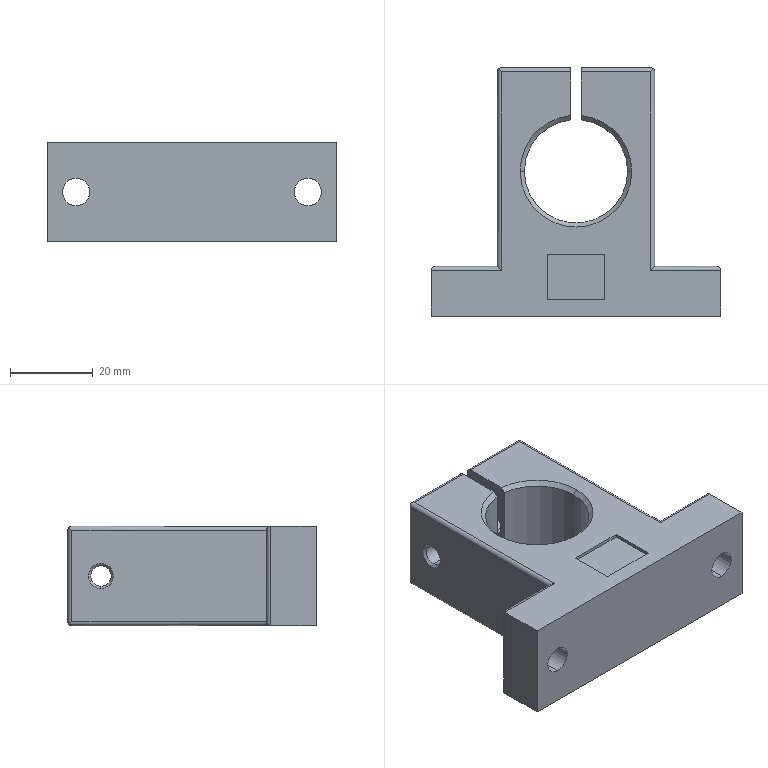Part | STEP file | SHAT25b | 1 solid | 58 faces | box 70 x 60 x 24 mm | volume 48947 mm3 | cylinder 29 | plane 19 | cone 10 | commonest cylinder face diameters 2 x16 6.6 x6 25 x3 4.917 x2 11 x2